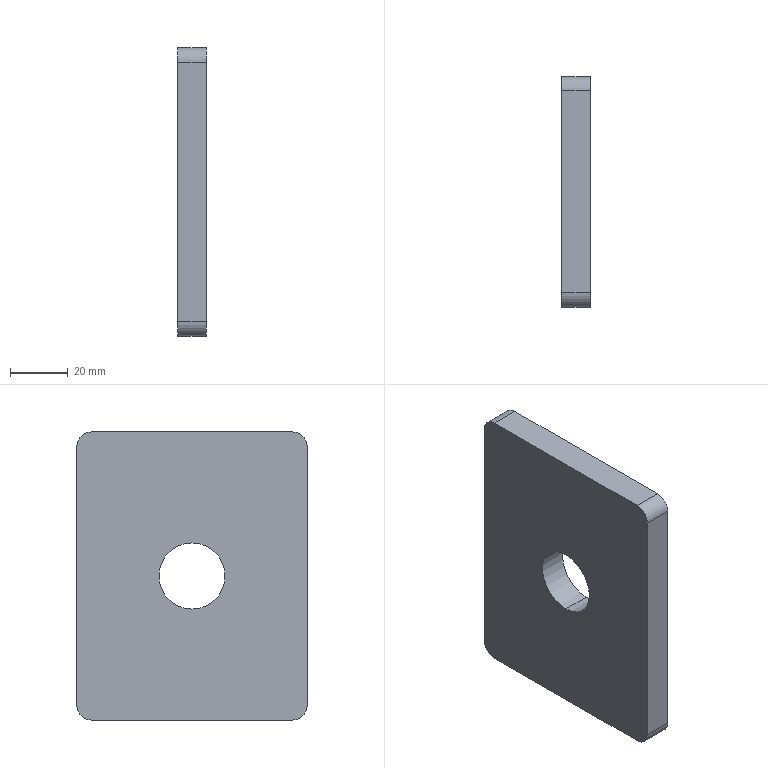Part | SolidWorks | features BaseBody 1 | 1 solid | 12 faces | box 10 x 80 x 100 mm | volume 75631 mm3 | cylinder 6 | plane 6 | commonest cylinder face diameters 10 x4 23 x2
STEP:
#1=CARTESIAN_POINT('',(5.,0.,11.5));
#2=VERTEX_POINT('',#1);
#3=CARTESIAN_POINT('',(5.,0.,-11.5));
#4=VERTEX_POINT('',#3);
#5=CARTESIAN_POINT('',(5.,0.,0.));
#6=DIRECTION('',(1.,0.,0.));
#7=DIRECTION('',(0.,0.,-1.));
#8=AXIS2_PLACEMENT_3D('',#5,#6,#7);
#9=CIRCLE('',#8,11.5);
#10=EDGE_CURVE('',#2,#4,#9,.T.);
#11=ORIENTED_EDGE('',*,*,#10,.T.);
#12=CARTESIAN_POINT('',(-5.,0.,-11.5));
#13=VERTEX_POINT('',#12);
#14=CARTESIAN_POINT('',(5.,0.,-11.5));
#15=DIRECTION('',(-1.,0.,0.));
#16=VECTOR('',#15,1000.);
#17=LINE('',#14,#16);
#18=EDGE_CURVE('',#4,#13,#17,.T.);
#19=ORIENTED_EDGE('',*,*,#18,.T.);
#20=CARTESIAN_POINT('',(-5.,0.,11.5));
#21=VERTEX_POINT('',#20);
#22=CARTESIAN_POINT('',(-5.,0.,0.));
#23=DIRECTION('',(1.,0.,0.));
#24=DIRECTION('',(0.,0.,-1.));
#25=AXIS2_PLACEMENT_3D('',#22,#23,#24);
#26=CIRCLE('',#25,11.5);
#27=EDGE_CURVE('',#21,#13,#26,.T.);
#28=ORIENTED_EDGE('',*,*,#27,.F.);
#29=CARTESIAN_POINT('',(5.,0.,11.5));
#30=DIRECTION('',(-1.,0.,0.));
#31=VECTOR('',#30,1000.);
#32=LINE('',#29,#31);
#33=EDGE_CURVE('',#2,#21,#32,.T.);
#34=ORIENTED_EDGE('',*,*,#33,.F.);
#35=EDGE_LOOP('',(#11,#19,#28,#34));
#36=FACE_OUTER_BOUND('',#35,.T.);
#37=CARTESIAN_POINT('',(5.,0.,0.));
#38=DIRECTION('',(-1.,0.,0.));
#39=DIRECTION('',(0.,0.,1.));
#40=AXIS2_PLACEMENT_3D('',#37,#38,#39);
#41=CYLINDRICAL_SURFACE('',#40,11.5);
#42=ADVANCED_FACE('',(#36),#41,.F.);
#43=CARTESIAN_POINT('',(5.,35.,-50.));
#44=VERTEX_POINT('',#43);
#45=CARTESIAN_POINT('',(5.,40.,-45.));
#46=VERTEX_POINT('',#45);
#47=CARTESIAN_POINT('',(5.,35.,-45.));
#48=DIRECTION('',(1.,0.,0.));
#49=DIRECTION('',(0.,0.,1.));
#50=AXIS2_PLACEMENT_3D('',#47,#48,#49);
#51=CIRCLE('',#50,5.);
#52=EDGE_CURVE('',#44,#46,#51,.T.);
#53=ORIENTED_EDGE('',*,*,#52,.T.);
#54=CARTESIAN_POINT('',(5.,40.,45.));
#55=VERTEX_POINT('',#54);
#56=CARTESIAN_POINT('',(5.,40.,45.));
#57=DIRECTION('',(0.,0.,1.));
#58=VECTOR('',#57,1000.);
#59=LINE('',#56,#58);
#60=EDGE_CURVE('',#46,#55,#59,.T.);
#61=ORIENTED_EDGE('',*,*,#60,.T.);
#62=CARTESIAN_POINT('',(5.,35.,50.));
#63=VERTEX_POINT('',#62);
#64=CARTESIAN_POINT('',(5.,35.,45.));
#65=DIRECTION('',(1.,0.,0.));
#66=DIRECTION('',(0.,0.,-1.));
#67=AXIS2_PLACEMENT_3D('',#64,#65,#66);
#68=CIRCLE('',#67,5.);
#69=EDGE_CURVE('',#55,#63,#68,.T.);
#70=ORIENTED_EDGE('',*,*,#69,.T.);
#71=CARTESIAN_POINT('',(5.,-35.,50.));
#72=VERTEX_POINT('',#71);
#73=CARTESIAN_POINT('',(5.,35.,50.));
#74=DIRECTION('',(0.,-1.,0.));
#75=VECTOR('',#74,1000.);
#76=LINE('',#73,#75);
#77=EDGE_CURVE('',#63,#72,#76,.T.);
#78=ORIENTED_EDGE('',*,*,#77,.T.);
#79=CARTESIAN_POINT('',(5.,-40.,45.));
#80=VERTEX_POINT('',#79);
#81=CARTESIAN_POINT('',(5.,-35.,45.));
#82=DIRECTION('',(1.,0.,0.));
#83=DIRECTION('',(0.,0.,-1.));
#84=AXIS2_PLACEMENT_3D('',#81,#82,#83);
#85=CIRCLE('',#84,5.);
#86=EDGE_CURVE('',#72,#80,#85,.T.);
#87=ORIENTED_EDGE('',*,*,#86,.T.);
#88=CARTESIAN_POINT('',(5.,-40.,-45.));
#89=VERTEX_POINT('',#88);
#90=CARTESIAN_POINT('',(5.,-40.,45.));
#91=DIRECTION('',(0.,0.,-1.));
#92=VECTOR('',#91,1000.);
#93=LINE('',#90,#92);
#94=EDGE_CURVE('',#80,#89,#93,.T.);
#95=ORIENTED_EDGE('',*,*,#94,.T.);
#96=CARTESIAN_POINT('',(5.,-35.,-50.));
#97=VERTEX_POINT('',#96);
#98=CARTESIAN_POINT('',(5.,-35.,-45.));
#99=DIRECTION('',(1.,0.,0.));
#100=DIRECTION('',(0.,0.,-1.));
#101=AXIS2_PLACEMENT_3D('',#98,#99,#100);
#102=CIRCLE('',#101,5.);
#103=EDGE_CURVE('',#89,#97,#102,.T.);
#104=ORIENTED_EDGE('',*,*,#103,.T.);
#105=CARTESIAN_POINT('',(5.,35.,-50.));
#106=DIRECTION('',(0.,1.,0.));
#107=VECTOR('',#106,1000.);
#108=LINE('',#105,#107);
#109=EDGE_CURVE('',#97,#44,#108,.T.);
#110=ORIENTED_EDGE('',*,*,#109,.T.);
#111=EDGE_LOOP('',(#53,#61,#70,#78,#87,#95,#104,#110));
#112=FACE_OUTER_BOUND('',#111,.T.);
#113=ORIENTED_EDGE('',*,*,#10,.F.);
#114=CARTESIAN_POINT('',(5.,0.,0.));
#115=DIRECTION('',(1.,0.,0.));
#116=DIRECTION('',(0.,0.,-1.));
#117=AXIS2_PLACEMENT_3D('',#114,#115,#116);
#118=CIRCLE('',#117,11.5);
#119=EDGE_CURVE('',#4,#2,#118,.T.);
#120=ORIENTED_EDGE('',*,*,#119,.F.);
#121=EDGE_LOOP('',(#113,#120));
#122=FACE_BOUND('',#121,.T.);
#123=CARTESIAN_POINT('',(5.,35.,-45.));
#124=DIRECTION('',(-1.,0.,0.));
#125=DIRECTION('',(0.,0.,1.));
#126=AXIS2_PLACEMENT_3D('',#123,#124,#125);
#127=PLANE('',#126);
#128=ADVANCED_FACE('',(#112,#122),#127,.F.);
#129=CARTESIAN_POINT('',(-5.,35.,-50.));
#130=VERTEX_POINT('',#129);
#131=CARTESIAN_POINT('',(-5.,40.,-45.));
#132=VERTEX_POINT('',#131);
#133=CARTESIAN_POINT('',(-5.,35.,-45.));
#134=DIRECTION('',(1.,0.,0.));
#135=DIRECTION('',(0.,0.,1.));
#136=AXIS2_PLACEMENT_3D('',#133,#134,#135);
#137=CIRCLE('',#136,5.);
#138=EDGE_CURVE('',#130,#132,#137,.T.);
#139=ORIENTED_EDGE('',*,*,#138,.F.);
#140=CARTESIAN_POINT('',(-5.,-35.,-50.));
#141=VERTEX_POINT('',#140);
#142=CARTESIAN_POINT('',(-5.,35.,-50.));
#143=DIRECTION('',(0.,1.,0.));
#144=VECTOR('',#143,1000.);
#145=LINE('',#142,#144);
#146=EDGE_CURVE('',#141,#130,#145,.T.);
#147=ORIENTED_EDGE('',*,*,#146,.F.);
#148=CARTESIAN_POINT('',(-5.,-40.,-45.));
#149=VERTEX_POINT('',#148);
#150=CARTESIAN_POINT('',(-5.,-35.,-45.));
#151=DIRECTION('',(1.,0.,0.));
#152=DIRECTION('',(0.,0.,-1.));
#153=AXIS2_PLACEMENT_3D('',#150,#151,#152);
#154=CIRCLE('',#153,5.);
#155=EDGE_CURVE('',#149,#141,#154,.T.);
#156=ORIENTED_EDGE('',*,*,#155,.F.);
#157=CARTESIAN_POINT('',(-5.,-40.,45.));
#158=VERTEX_POINT('',#157);
#159=CARTESIAN_POINT('',(-5.,-40.,45.));
#160=DIRECTION('',(0.,0.,-1.));
#161=VECTOR('',#160,1000.);
#162=LINE('',#159,#161);
#163=EDGE_CURVE('',#158,#149,#162,.T.);
#164=ORIENTED_EDGE('',*,*,#163,.F.);
#165=CARTESIAN_POINT('',(-5.,-35.,50.));
#166=VERTEX_POINT('',#165);
#167=CARTESIAN_POINT('',(-5.,-35.,45.));
#168=DIRECTION('',(1.,0.,0.));
#169=DIRECTION('',(0.,0.,-1.));
#170=AXIS2_PLACEMENT_3D('',#167,#168,#169);
#171=CIRCLE('',#170,5.);
#172=EDGE_CURVE('',#166,#158,#171,.T.);
#173=ORIENTED_EDGE('',*,*,#172,.F.);
#174=CARTESIAN_POINT('',(-5.,35.,50.));
#175=VERTEX_POINT('',#174);
#176=CARTESIAN_POINT('',(-5.,35.,50.));
#177=DIRECTION('',(0.,-1.,0.));
#178=VECTOR('',#177,1000.);
#179=LINE('',#176,#178);
#180=EDGE_CURVE('',#175,#166,#179,.T.);
#181=ORIENTED_EDGE('',*,*,#180,.F.);
#182=CARTESIAN_POINT('',(-5.,40.,45.));
#183=VERTEX_POINT('',#182);
#184=CARTESIAN_POINT('',(-5.,35.,45.));
#185=DIRECTION('',(1.,0.,0.));
#186=DIRECTION('',(0.,0.,-1.));
#187=AXIS2_PLACEMENT_3D('',#184,#185,#186);
#188=CIRCLE('',#187,5.);
#189=EDGE_CURVE('',#183,#175,#188,.T.);
#190=ORIENTED_EDGE('',*,*,#189,.F.);
#191=CARTESIAN_POINT('',(-5.,40.,45.));
#192=DIRECTION('',(0.,0.,1.));
#193=VECTOR('',#192,1000.);
#194=LINE('',#191,#193);
#195=EDGE_CURVE('',#132,#183,#194,.T.);
#196=ORIENTED_EDGE('',*,*,#195,.F.);
#197=EDGE_LOOP('',(#139,#147,#156,#164,#173,#181,#190,#196));
#198=FACE_OUTER_BOUND('',#197,.T.);
#199=ORIENTED_EDGE('',*,*,#27,.T.);
#200=CARTESIAN_POINT('',(-5.,0.,0.));
#201=DIRECTION('',(1.,0.,0.));
#202=DIRECTION('',(0.,0.,-1.));
#203=AXIS2_PLACEMENT_3D('',#200,#201,#202);
#204=CIRCLE('',#203,11.5);
#205=EDGE_CURVE('',#13,#21,#204,.T.);
#206=ORIENTED_EDGE('',*,*,#205,.T.);
#207=EDGE_LOOP('',(#199,#206));
#208=FACE_BOUND('',#207,.T.);
#209=CARTESIAN_POINT('',(-5.,35.,-45.));
#210=DIRECTION('',(-1.,0.,0.));
#211=DIRECTION('',(0.,0.,1.));
#212=AXIS2_PLACEMENT_3D('',#209,#210,#211);
#213=PLANE('',#212);
#214=ADVANCED_FACE('',(#198,#208),#213,.T.);
#215=ORIENTED_EDGE('',*,*,#138,.T.);
#216=CARTESIAN_POINT('',(5.,40.,-45.));
#217=DIRECTION('',(-1.,0.,0.));
#218=VECTOR('',#217,1000.);
#219=LINE('',#216,#218);
#220=EDGE_CURVE('',#46,#132,#219,.T.);
#221=ORIENTED_EDGE('',*,*,#220,.F.);
#222=ORIENTED_EDGE('',*,*,#52,.F.);
#223=CARTESIAN_POINT('',(5.,35.,-50.));
#224=DIRECTION('',(-1.,0.,0.));
#225=VECTOR('',#224,1000.);
#226=LINE('',#223,#225);
#227=EDGE_CURVE('',#44,#130,#226,.T.);
#228=ORIENTED_EDGE('',*,*,#227,.T.);
#229=EDGE_LOOP('',(#215,#221,#222,#228));
#230=FACE_OUTER_BOUND('',#229,.T.);
#231=CARTESIAN_POINT('',(5.,35.,-45.));
#232=DIRECTION('',(-1.,0.,0.));
#233=DIRECTION('',(0.,0.,1.));
#234=AXIS2_PLACEMENT_3D('',#231,#232,#233);
#235=CYLINDRICAL_SURFACE('',#234,5.);
#236=ADVANCED_FACE('',(#230),#235,.T.);
#237=ORIENTED_EDGE('',*,*,#195,.T.);
#238=CARTESIAN_POINT('',(5.,40.,45.));
#239=DIRECTION('',(-1.,0.,0.));
#240=VECTOR('',#239,1000.);
#241=LINE('',#238,#240);
#242=EDGE_CURVE('',#55,#183,#241,.T.);
#243=ORIENTED_EDGE('',*,*,#242,.F.);
#244=ORIENTED_EDGE('',*,*,#60,.F.);
#245=ORIENTED_EDGE('',*,*,#220,.T.);
#246=EDGE_LOOP('',(#237,#243,#244,#245));
#247=FACE_OUTER_BOUND('',#246,.T.);
#248=CARTESIAN_POINT('',(5.,40.,45.));
#249=DIRECTION('',(0.,-1.,0.));
#250=DIRECTION('',(0.,0.,-1.));
#251=AXIS2_PLACEMENT_3D('',#248,#249,#250);
#252=PLANE('',#251);
#253=ADVANCED_FACE('',(#247),#252,.F.);
#254=ORIENTED_EDGE('',*,*,#189,.T.);
#255=CARTESIAN_POINT('',(5.,35.,50.));
#256=DIRECTION('',(-1.,0.,0.));
#257=VECTOR('',#256,1000.);
#258=LINE('',#255,#257);
#259=EDGE_CURVE('',#63,#175,#258,.T.);
#260=ORIENTED_EDGE('',*,*,#259,.F.);
#261=ORIENTED_EDGE('',*,*,#69,.F.);
#262=ORIENTED_EDGE('',*,*,#242,.T.);
#263=EDGE_LOOP('',(#254,#260,#261,#262));
#264=FACE_OUTER_BOUND('',#263,.T.);
#265=CARTESIAN_POINT('',(5.,35.,45.));
#266=DIRECTION('',(-1.,0.,0.));
#267=DIRECTION('',(0.,0.,1.));
#268=AXIS2_PLACEMENT_3D('',#265,#266,#267);
#269=CYLINDRICAL_SURFACE('',#268,5.);
#270=ADVANCED_FACE('',(#264),#269,.T.);
#271=ORIENTED_EDGE('',*,*,#180,.T.);
#272=CARTESIAN_POINT('',(5.,-35.,50.));
#273=DIRECTION('',(-1.,0.,0.));
#274=VECTOR('',#273,1000.);
#275=LINE('',#272,#274);
#276=EDGE_CURVE('',#72,#166,#275,.T.);
#277=ORIENTED_EDGE('',*,*,#276,.F.);
#278=ORIENTED_EDGE('',*,*,#77,.F.);
#279=ORIENTED_EDGE('',*,*,#259,.T.);
#280=EDGE_LOOP('',(#271,#277,#278,#279));
#281=FACE_OUTER_BOUND('',#280,.T.);
#282=CARTESIAN_POINT('',(5.,35.,50.));
#283=DIRECTION('',(0.,0.,-1.));
#284=DIRECTION('',(0.,1.,0.));
#285=AXIS2_PLACEMENT_3D('',#282,#283,#284);
#286=PLANE('',#285);
#287=ADVANCED_FACE('',(#281),#286,.F.);
#288=ORIENTED_EDGE('',*,*,#172,.T.);
#289=CARTESIAN_POINT('',(5.,-40.,45.));
#290=DIRECTION('',(-1.,0.,0.));
#291=VECTOR('',#290,1000.);
#292=LINE('',#289,#291);
#293=EDGE_CURVE('',#80,#158,#292,.T.);
#294=ORIENTED_EDGE('',*,*,#293,.F.);
#295=ORIENTED_EDGE('',*,*,#86,.F.);
#296=ORIENTED_EDGE('',*,*,#276,.T.);
#297=EDGE_LOOP('',(#288,#294,#295,#296));
#298=FACE_OUTER_BOUND('',#297,.T.);
#299=CARTESIAN_POINT('',(5.,-35.,45.));
#300=DIRECTION('',(-1.,0.,0.));
#301=DIRECTION('',(0.,0.,1.));
#302=AXIS2_PLACEMENT_3D('',#299,#300,#301);
#303=CYLINDRICAL_SURFACE('',#302,5.);
#304=ADVANCED_FACE('',(#298),#303,.T.);
#305=ORIENTED_EDGE('',*,*,#163,.T.);
#306=CARTESIAN_POINT('',(5.,-40.,-45.));
#307=DIRECTION('',(-1.,0.,0.));
#308=VECTOR('',#307,1000.);
#309=LINE('',#306,#308);
#310=EDGE_CURVE('',#89,#149,#309,.T.);
#311=ORIENTED_EDGE('',*,*,#310,.F.);
#312=ORIENTED_EDGE('',*,*,#94,.F.);
#313=ORIENTED_EDGE('',*,*,#293,.T.);
#314=EDGE_LOOP('',(#305,#311,#312,#313));
#315=FACE_OUTER_BOUND('',#314,.T.);
#316=CARTESIAN_POINT('',(5.,-40.,45.));
#317=DIRECTION('',(0.,1.,0.));
#318=DIRECTION('',(0.,0.,1.));
#319=AXIS2_PLACEMENT_3D('',#316,#317,#318);
#320=PLANE('',#319);
#321=ADVANCED_FACE('',(#315),#320,.F.);
#322=ORIENTED_EDGE('',*,*,#155,.T.);
#323=CARTESIAN_POINT('',(5.,-35.,-50.));
#324=DIRECTION('',(-1.,0.,0.));
#325=VECTOR('',#324,1000.);
#326=LINE('',#323,#325);
#327=EDGE_CURVE('',#97,#141,#326,.T.);
#328=ORIENTED_EDGE('',*,*,#327,.F.);
#329=ORIENTED_EDGE('',*,*,#103,.F.);
#330=ORIENTED_EDGE('',*,*,#310,.T.);
#331=EDGE_LOOP('',(#322,#328,#329,#330));
#332=FACE_OUTER_BOUND('',#331,.T.);
#333=CARTESIAN_POINT('',(5.,-35.,-45.));
#334=DIRECTION('',(-1.,0.,0.));
#335=DIRECTION('',(0.,0.,1.));
#336=AXIS2_PLACEMENT_3D('',#333,#334,#335);
#337=CYLINDRICAL_SURFACE('',#336,5.);
#338=ADVANCED_FACE('',(#332),#337,.T.);
#339=ORIENTED_EDGE('',*,*,#146,.T.);
#340=ORIENTED_EDGE('',*,*,#227,.F.);
#341=ORIENTED_EDGE('',*,*,#109,.F.);
#342=ORIENTED_EDGE('',*,*,#327,.T.);
#343=EDGE_LOOP('',(#339,#340,#341,#342));
#344=FACE_OUTER_BOUND('',#343,.T.);
#345=CARTESIAN_POINT('',(5.,35.,-50.));
#346=DIRECTION('',(0.,0.,1.));
#347=DIRECTION('',(0.,-1.,0.));
#348=AXIS2_PLACEMENT_3D('',#345,#346,#347);
#349=PLANE('',#348);
#350=ADVANCED_FACE('',(#344),#349,.F.);
#351=ORIENTED_EDGE('',*,*,#18,.F.);
#352=ORIENTED_EDGE('',*,*,#119,.T.);
#353=ORIENTED_EDGE('',*,*,#33,.T.);
#354=ORIENTED_EDGE('',*,*,#205,.F.);
#355=EDGE_LOOP('',(#351,#352,#353,#354));
#356=FACE_OUTER_BOUND('',#355,.T.);
#357=CARTESIAN_POINT('',(5.,0.,0.));
#358=DIRECTION('',(-1.,0.,0.));
#359=DIRECTION('',(0.,0.,1.));
#360=AXIS2_PLACEMENT_3D('',#357,#358,#359);
#361=CYLINDRICAL_SURFACE('',#360,11.5);
#362=ADVANCED_FACE('',(#356),#361,.F.);
#363=CLOSED_SHELL('',(#42,#128,#214,#236,#253,#270,#287,#304,#321,#338,#350,#362));
#364=MANIFOLD_SOLID_BREP('',#363);
#365=CARTESIAN_POINT('',(0.,0.,0.));
#366=DIRECTION('',(0.,0.,1.));
#367=DIRECTION('',(1.,0.,0.));
#368=AXIS2_PLACEMENT_3D('',#365,#366,#367);
#369=(LENGTH_UNIT()NAMED_UNIT(*)SI_UNIT(.MILLI.,.METRE.));
#370=UNCERTAINTY_MEASURE_WITH_UNIT(LENGTH_MEASURE(0.00001),#369,'','');
#371=(NAMED_UNIT(*)PLANE_ANGLE_UNIT()SI_UNIT($,.RADIAN.));
#372=(NAMED_UNIT(*)SI_UNIT($,.STERADIAN.)SOLID_ANGLE_UNIT());
#373=(GEOMETRIC_REPRESENTATION_CONTEXT(3)GLOBAL_UNCERTAINTY_ASSIGNED_CONTEXT((#370))GLOBAL_UNIT_ASSIGNED_CONTEXT((#369,#371,#372))REPRESENTATION_CONTEXT('',''));
#374=ADVANCED_BREP_SHAPE_REPRESENTATION('',(#364,#368),#373);